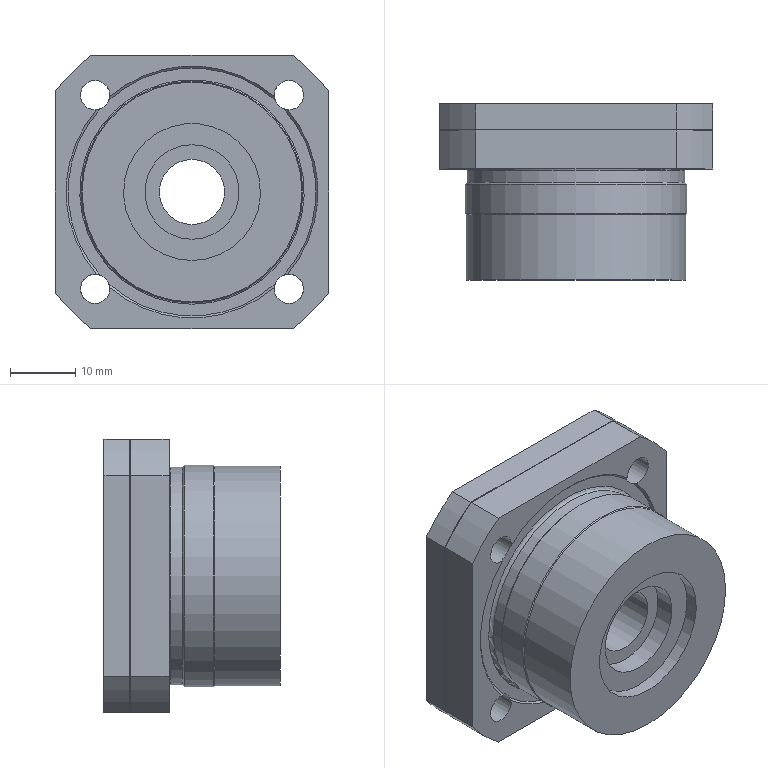Part | STEP file | ROTATION MC_NEW VER-0610_489 | 1 solid | 105 faces | box 42 x 27 x 42 mm | volume 26913 mm3 | plane 62 | cylinder 35 | cone 7 | torus 1 | commonest cylinder face diameters 52 x8 4.5 x4 6.2 x4 7 x4 8 x4 51.9 x4